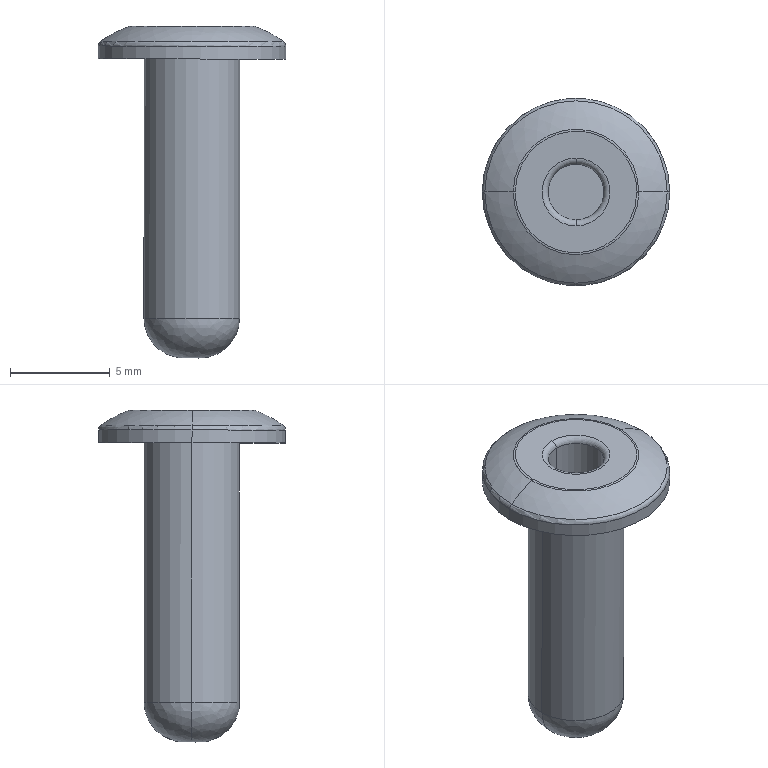Part | SolidWorks | features BaseBody 1 | 1 solid | 22 faces | box 9.401 x 9.4 x 16.653 mm | volume 328.564 mm3 | torus 8 | cylinder 6 | spline 4 | plane 4 | commonest cylinder face diameters 2.8 x2 4.8 x2 9.4 x2
STEP:
#1=CARTESIAN_POINT('',(200.964,12.529,-10.322));
#2=VERTEX_POINT('',#1);
#3=CARTESIAN_POINT('',(200.837,12.529,-10.077));
#4=VERTEX_POINT('',#3);
#5=CARTESIAN_POINT('',(200.664,12.529,-10.322));
#6=DIRECTION('',(0.00003827,-1.,-0.0004455));
#7=DIRECTION('',(1.,0.00003864,-0.0008339));
#8=AXIS2_PLACEMENT_3D('',#5,#6,#7);
#9=CIRCLE('',#8,0.3);
#10=EDGE_CURVE('',#2,#4,#9,.T.);
#11=ORIENTED_EDGE('',*,*,#10,.T.);
#12=CARTESIAN_POINT('',(191.692,12.529,-10.069));
#13=VERTEX_POINT('',#12);
#14=CARTESIAN_POINT('',(196.265,12.529,-10.073));
#15=DIRECTION('',(-0.0008339,0.0004454,-1.));
#16=DIRECTION('',(1.,0.00002965,-0.0008339));
#17=AXIS2_PLACEMENT_3D('',#14,#15,#16);
#18=CIRCLE('',#17,4.573);
#19=EDGE_CURVE('',#4,#13,#18,.T.);
#20=ORIENTED_EDGE('',*,*,#19,.T.);
#21=CARTESIAN_POINT('',(191.564,12.529,-10.315));
#22=VERTEX_POINT('',#21);
#23=CARTESIAN_POINT('',(191.864,12.529,-10.315));
#24=DIRECTION('',(-0.00003827,1.,0.0004455));
#25=DIRECTION('',(-1.,-0.00003864,0.0008339));
#26=AXIS2_PLACEMENT_3D('',#23,#24,#25);
#27=CIRCLE('',#26,0.3);
#28=EDGE_CURVE('',#22,#13,#27,.T.);
#29=ORIENTED_EDGE('',*,*,#28,.F.);
#30=CARTESIAN_POINT('',(196.264,12.529,-10.318));
#31=DIRECTION('',(-0.0008339,0.0004454,-1.));
#32=DIRECTION('',(-1.,-0.007345,0.0008306));
#33=AXIS2_PLACEMENT_3D('',#30,#31,#32);
#34=CIRCLE('',#33,4.7);
#35=EDGE_CURVE('',#2,#22,#34,.T.);
#36=ORIENTED_EDGE('',*,*,#35,.F.);
#37=EDGE_LOOP('',(#11,#20,#29,#36));
#38=FACE_OUTER_BOUND('',#37,.T.);
#39=CARTESIAN_POINT('',(196.264,12.529,-10.318));
#40=DIRECTION('',(-0.0008339,0.0004454,-1.));
#41=DIRECTION('',(1.,0.007345,-0.0008306));
#42=AXIS2_PLACEMENT_3D('',#39,#40,#41);
#43=TOROIDAL_SURFACE('',#42,4.4,0.3);
#44=ADVANCED_FACE('',(#38),#43,.T.);
#45=CARTESIAN_POINT('',(191.564,12.529,-10.961));
#46=VERTEX_POINT('',#45);
#47=CARTESIAN_POINT('',(200.964,12.529,-10.969));
#48=VERTEX_POINT('',#47);
#49=CARTESIAN_POINT('',(196.264,12.529,-10.965));
#50=DIRECTION('',(0.0008339,-0.0004454,1.));
#51=DIRECTION('',(-1.,-0.00003864,0.0008339));
#52=AXIS2_PLACEMENT_3D('',#49,#50,#51);
#53=CIRCLE('',#52,4.7);
#54=EDGE_CURVE('',#46,#48,#53,.T.);
#55=ORIENTED_EDGE('',*,*,#54,.T.);
#56=CARTESIAN_POINT('',(200.964,12.529,-10.322));
#57=DIRECTION('',(-0.0008339,0.0004454,-1.));
#58=VECTOR('',#57,1000.);
#59=LINE('',#56,#58);
#60=EDGE_CURVE('',#2,#48,#59,.T.);
#61=ORIENTED_EDGE('',*,*,#60,.F.);
#62=ORIENTED_EDGE('',*,*,#35,.T.);
#63=CARTESIAN_POINT('',(191.564,12.529,-10.315));
#64=DIRECTION('',(-0.0008339,0.0004454,-1.));
#65=VECTOR('',#64,1000.);
#66=LINE('',#63,#65);
#67=EDGE_CURVE('',#22,#46,#66,.T.);
#68=ORIENTED_EDGE('',*,*,#67,.T.);
#69=EDGE_LOOP('',(#55,#61,#62,#68));
#70=FACE_OUTER_BOUND('',#69,.T.);
#71=CARTESIAN_POINT('',(196.265,12.529,-9.315));
#72=DIRECTION('',(-0.0008339,0.0004454,-1.));
#73=DIRECTION('',(1.,0.00003864,-0.0008339));
#74=AXIS2_PLACEMENT_3D('',#71,#72,#73);
#75=CYLINDRICAL_SURFACE('',#74,4.7);
#76=ADVANCED_FACE('',(#70),#75,.T.);
#77=CARTESIAN_POINT('',(196.264,12.529,-10.965));
#78=DIRECTION('',(0.0008339,-0.0004454,1.));
#79=DIRECTION('',(1.,0.00003864,-0.0008339));
#80=AXIS2_PLACEMENT_3D('',#77,#78,#79);
#81=CIRCLE('',#80,4.7);
#82=EDGE_CURVE('',#48,#46,#81,.T.);
#83=ORIENTED_EDGE('',*,*,#82,.T.);
#84=ORIENTED_EDGE('',*,*,#67,.F.);
#85=CARTESIAN_POINT('',(196.264,12.529,-10.318));
#86=DIRECTION('',(-0.0008339,0.0004454,-1.));
#87=DIRECTION('',(-1.,-0.00003864,0.0008339));
#88=AXIS2_PLACEMENT_3D('',#85,#86,#87);
#89=CIRCLE('',#88,4.7);
#90=EDGE_CURVE('',#22,#2,#89,.T.);
#91=ORIENTED_EDGE('',*,*,#90,.T.);
#92=ORIENTED_EDGE('',*,*,#60,.T.);
#93=EDGE_LOOP('',(#83,#84,#91,#92));
#94=FACE_OUTER_BOUND('',#93,.T.);
#95=CARTESIAN_POINT('',(196.265,12.529,-9.315));
#96=DIRECTION('',(-0.0008339,0.0004454,-1.));
#97=DIRECTION('',(1.,0.00003864,-0.0008339));
#98=AXIS2_PLACEMENT_3D('',#95,#96,#97);
#99=CYLINDRICAL_SURFACE('',#98,4.7);
#100=ADVANCED_FACE('',(#94),#99,.T.);
#101=ORIENTED_EDGE('',*,*,#28,.T.);
#102=CARTESIAN_POINT('',(196.265,12.529,-10.073));
#103=DIRECTION('',(-0.0008339,0.0004454,-1.));
#104=DIRECTION('',(-1.,-0.00002965,0.0008339));
#105=AXIS2_PLACEMENT_3D('',#102,#103,#104);
#106=CIRCLE('',#105,4.573);
#107=EDGE_CURVE('',#13,#4,#106,.T.);
#108=ORIENTED_EDGE('',*,*,#107,.T.);
#109=ORIENTED_EDGE('',*,*,#10,.F.);
#110=ORIENTED_EDGE('',*,*,#90,.F.);
#111=EDGE_LOOP('',(#101,#108,#109,#110));
#112=FACE_OUTER_BOUND('',#111,.T.);
#113=CARTESIAN_POINT('',(196.264,12.529,-10.318));
#114=DIRECTION('',(-0.0008339,0.0004454,-1.));
#115=DIRECTION('',(-1.,-0.007345,0.0008306));
#116=AXIS2_PLACEMENT_3D('',#113,#114,#115);
#117=TOROIDAL_SURFACE('',#116,4.4,0.3);
#118=ADVANCED_FACE('',(#112),#117,.T.);
#119=CARTESIAN_POINT('',(199.415,12.529,-9.336));
#120=VERTEX_POINT('',#119);
#121=CARTESIAN_POINT('',(200.837,12.529,-10.077));
#122=CARTESIAN_POINT('',(200.691,12.529,-9.974));
#123=CARTESIAN_POINT('',(200.39,12.529,-9.781));
#124=CARTESIAN_POINT('',(199.915,12.529,-9.533));
#125=CARTESIAN_POINT('',(199.584,12.529,-9.396));
#126=CARTESIAN_POINT('',(199.415,12.529,-9.336));
#127=B_SPLINE_CURVE_WITH_KNOTS('',3,(#121,#122,#123,#124,#125,#126),.UNSPECIFIED.,.F.,.F.,(4,1,1,4),(0.000000006,0.3333,0.6667,1.),.UNSPECIFIED.);
#128=EDGE_CURVE('',#4,#120,#127,.T.);
#129=ORIENTED_EDGE('',*,*,#128,.F.);
#130=ORIENTED_EDGE('',*,*,#107,.F.);
#131=CARTESIAN_POINT('',(193.115,12.528,-9.33));
#132=VERTEX_POINT('',#131);
#133=CARTESIAN_POINT('',(191.692,12.529,-10.069));
#134=CARTESIAN_POINT('',(191.838,12.529,-9.967));
#135=CARTESIAN_POINT('',(192.139,12.529,-9.774));
#136=CARTESIAN_POINT('',(192.616,12.529,-9.527));
#137=CARTESIAN_POINT('',(192.947,12.528,-9.391));
#138=CARTESIAN_POINT('',(193.115,12.528,-9.33));
#139=B_SPLINE_CURVE_WITH_KNOTS('',3,(#133,#134,#135,#136,#137,#138),.UNSPECIFIED.,.F.,.F.,(4,1,1,4),(0.000001822,0.3333,0.6667,1.),.UNSPECIFIED.);
#140=EDGE_CURVE('',#13,#132,#139,.T.);
#141=ORIENTED_EDGE('',*,*,#140,.T.);
#142=CARTESIAN_POINT('',(193.116,12.566,-9.33));
#143=VERTEX_POINT('',#142);
#144=CARTESIAN_POINT('',(196.265,12.529,-9.333));
#145=DIRECTION('',(0.0008339,-0.0004454,1.));
#146=DIRECTION('',(-0.9999,0.01201,0.0008392));
#147=AXIS2_PLACEMENT_3D('',#144,#145,#146);
#148=CIRCLE('',#147,3.15);
#149=EDGE_CURVE('',#143,#132,#148,.T.);
#150=ORIENTED_EDGE('',*,*,#149,.F.);
#151=CARTESIAN_POINT('',(196.265,12.529,-9.333));
#152=DIRECTION('',(0.0008339,-0.0004454,1.));
#153=DIRECTION('',(-0.9999,0.01201,0.0008392));
#154=AXIS2_PLACEMENT_3D('',#151,#152,#153);
#155=CIRCLE('',#154,3.15);
#156=EDGE_CURVE('',#120,#143,#155,.T.);
#157=ORIENTED_EDGE('',*,*,#156,.F.);
#158=EDGE_LOOP('',(#129,#130,#141,#150,#157));
#159=FACE_OUTER_BOUND('',#158,.T.);
#160=CARTESIAN_POINT('',(193.235,12.338,-9.291));
#161=CARTESIAN_POINT('',(192.65,12.301,-9.489));
#162=CARTESIAN_POINT('',(192.102,12.267,-9.774));
#163=CARTESIAN_POINT('',(191.604,12.235,-10.14));
#164=CARTESIAN_POINT('',(193.117,14.203,-9.29));
#165=CARTESIAN_POINT('',(192.509,14.526,-9.487));
#166=CARTESIAN_POINT('',(191.94,14.829,-9.772));
#167=CARTESIAN_POINT('',(191.423,15.104,-10.138));
#168=CARTESIAN_POINT('',(194.396,15.565,-9.291));
#169=CARTESIAN_POINT('',(194.036,16.151,-9.488));
#170=CARTESIAN_POINT('',(193.698,16.7,-9.773));
#171=CARTESIAN_POINT('',(193.39,17.199,-10.139));
#172=CARTESIAN_POINT('',(196.265,15.565,-9.292));
#173=CARTESIAN_POINT('',(196.265,16.151,-9.49));
#174=CARTESIAN_POINT('',(196.265,16.7,-9.775));
#175=CARTESIAN_POINT('',(196.264,17.199,-10.141));
#176=CARTESIAN_POINT('',(198.134,15.565,-9.294));
#177=CARTESIAN_POINT('',(198.495,16.151,-9.492));
#178=CARTESIAN_POINT('',(198.832,16.7,-9.777));
#179=CARTESIAN_POINT('',(199.138,17.199,-10.144));
#180=CARTESIAN_POINT('',(199.413,14.203,-9.295));
#181=CARTESIAN_POINT('',(200.021,14.526,-9.494));
#182=CARTESIAN_POINT('',(200.589,14.829,-9.78));
#183=CARTESIAN_POINT('',(201.106,15.104,-10.146));
#184=CARTESIAN_POINT('',(199.296,12.338,-9.296));
#185=CARTESIAN_POINT('',(199.881,12.301,-9.495));
#186=CARTESIAN_POINT('',(200.428,12.267,-9.781));
#187=CARTESIAN_POINT('',(200.926,12.236,-10.147));
#188=(BOUNDED_SURFACE()B_SPLINE_SURFACE(3,3,((#160,#161,#162,#163),(#164,#165,#166,#167),(#168,#169,#170,#171),(#172,#173,#174,#175),(#176,#177,#178,#179),(#180,#181,#182,#183),(#184,#185,#186,#187)),.UNSPECIFIED.,.F.,.F.,.F.)B_SPLINE_SURFACE_WITH_KNOTS((4,3,4),(4,4),(0.,1.,2.),(0.,1.),.UNSPECIFIED.)GEOMETRIC_REPRESENTATION_ITEM()RATIONAL_B_SPLINE_SURFACE(((1.194,1.185,1.185,1.194),(0.9432,0.9357,0.9357,0.9432),(0.9432,0.9357,0.9357,0.9432),(1.194,1.185,1.185,1.194),(0.9432,0.9357,0.9357,0.9432),(0.9432,0.9357,0.9357,0.9432),(1.194,1.185,1.185,1.194)))REPRESENTATION_ITEM('')SURFACE());
#189=ADVANCED_FACE('',(#159),#188,.T.);
#190=CARTESIAN_POINT('',(193.216,12.565,-9.313));
#191=VERTEX_POINT('',#190);
#192=CARTESIAN_POINT('',(193.217,12.565,-9.613));
#193=DIRECTION('',(-0.01201,-0.9999,-0.0004354));
#194=DIRECTION('',(0.9999,-0.01201,0.));
#195=AXIS2_PLACEMENT_3D('',#192,#193,#194);
#196=CIRCLE('',#195,0.3);
#197=EDGE_CURVE('',#191,#143,#196,.T.);
#198=ORIENTED_EDGE('',*,*,#197,.F.);
#199=CARTESIAN_POINT('',(199.315,12.527,-9.318));
#200=VERTEX_POINT('',#199);
#201=CARTESIAN_POINT('',(193.216,12.565,-9.313));
#202=CARTESIAN_POINT('',(193.221,12.711,-9.313));
#203=CARTESIAN_POINT('',(193.234,12.911,-9.313));
#204=CARTESIAN_POINT('',(193.298,13.218,-9.313));
#205=CARTESIAN_POINT('',(193.313,13.284,-9.313));
#206=CARTESIAN_POINT('',(193.345,13.401,-9.313));
#207=CARTESIAN_POINT('',(193.362,13.456,-9.313));
#208=CARTESIAN_POINT('',(193.414,13.612,-9.313));
#209=CARTESIAN_POINT('',(193.45,13.702,-9.313));
#210=CARTESIAN_POINT('',(193.502,13.817,-9.312));
#211=CARTESIAN_POINT('',(193.519,13.853,-9.312));
#212=CARTESIAN_POINT('',(193.539,13.893,-9.312));
#213=CARTESIAN_POINT('',(193.543,13.902,-9.312));
#214=CARTESIAN_POINT('',(193.554,13.924,-9.312));
#215=CARTESIAN_POINT('',(193.571,13.956,-9.312));
#216=CARTESIAN_POINT('',(193.635,14.074,-9.312));
#217=CARTESIAN_POINT('',(193.699,14.178,-9.312));
#218=CARTESIAN_POINT('',(193.783,14.299,-9.313));
#219=CARTESIAN_POINT('',(193.826,14.358,-9.313));
#220=CARTESIAN_POINT('',(193.871,14.416,-9.313));
#221=CARTESIAN_POINT('',(193.894,14.444,-9.313));
#222=CARTESIAN_POINT('',(193.904,14.456,-9.313));
#223=CARTESIAN_POINT('',(193.913,14.467,-9.313));
#224=CARTESIAN_POINT('',(193.917,14.472,-9.313));
#225=CARTESIAN_POINT('',(193.961,14.524,-9.313));
#226=CARTESIAN_POINT('',(194.013,14.584,-9.313));
#227=CARTESIAN_POINT('',(194.149,14.724,-9.313));
#228=CARTESIAN_POINT('',(194.233,14.804,-9.313));
#229=CARTESIAN_POINT('',(194.351,14.9,-9.313));
#230=CARTESIAN_POINT('',(194.365,14.911,-9.313));
#231=CARTESIAN_POINT('',(194.385,14.927,-9.313));
#232=CARTESIAN_POINT('',(194.389,14.93,-9.313));
#233=CARTESIAN_POINT('',(194.398,14.937,-9.313));
#234=CARTESIAN_POINT('',(194.42,14.954,-9.313));
#235=CARTESIAN_POINT('',(194.477,14.997,-9.313));
#236=CARTESIAN_POINT('',(194.533,15.036,-9.313));
#237=CARTESIAN_POINT('',(194.724,15.165,-9.313));
#238=CARTESIAN_POINT('',(194.897,15.26,-9.313));
#239=CARTESIAN_POINT('',(195.135,15.36,-9.313));
#240=CARTESIAN_POINT('',(195.184,15.38,-9.313));
#241=CARTESIAN_POINT('',(195.241,15.4,-9.313));
#242=CARTESIAN_POINT('',(195.247,15.402,-9.313));
#243=CARTESIAN_POINT('',(195.26,15.407,-9.313));
#244=CARTESIAN_POINT('',(195.258,15.406,-9.313));
#245=CARTESIAN_POINT('',(195.263,15.408,-9.313));
#246=CARTESIAN_POINT('',(195.275,15.412,-9.313));
#247=CARTESIAN_POINT('',(195.293,15.418,-9.313));
#248=CARTESIAN_POINT('',(195.364,15.442,-9.313));
#249=CARTESIAN_POINT('',(195.464,15.474,-9.313));
#250=CARTESIAN_POINT('',(195.679,15.521,-9.314));
#251=CARTESIAN_POINT('',(195.768,15.537,-9.314));
#252=CARTESIAN_POINT('',(195.914,15.557,-9.314));
#253=CARTESIAN_POINT('',(195.979,15.563,-9.314));
#254=CARTESIAN_POINT('',(196.088,15.571,-9.314));
#255=CARTESIAN_POINT('',(196.133,15.573,-9.314));
#256=CARTESIAN_POINT('',(196.186,15.575,-9.314));
#257=CARTESIAN_POINT('',(196.201,15.575,-9.314));
#258=CARTESIAN_POINT('',(196.227,15.576,-9.314));
#259=CARTESIAN_POINT('',(196.238,15.576,-9.314));
#260=CARTESIAN_POINT('',(196.273,15.576,-9.314));
#261=CARTESIAN_POINT('',(196.336,15.577,-9.314));
#262=CARTESIAN_POINT('',(196.484,15.569,-9.314));
#263=CARTESIAN_POINT('',(196.542,15.564,-9.314));
#264=CARTESIAN_POINT('',(196.643,15.553,-9.314));
#265=CARTESIAN_POINT('',(196.678,15.549,-9.314));
#266=CARTESIAN_POINT('',(196.735,15.54,-9.314));
#267=CARTESIAN_POINT('',(196.764,15.536,-9.314));
#268=CARTESIAN_POINT('',(196.799,15.53,-9.314));
#269=CARTESIAN_POINT('',(196.817,15.526,-9.314));
#270=CARTESIAN_POINT('',(196.825,15.525,-9.315));
#271=CARTESIAN_POINT('',(196.83,15.524,-9.315));
#272=CARTESIAN_POINT('',(196.834,15.523,-9.315));
#273=CARTESIAN_POINT('',(196.93,15.505,-9.315));
#274=CARTESIAN_POINT('',(197.025,15.483,-9.315));
#275=CARTESIAN_POINT('',(197.167,15.441,-9.315));
#276=CARTESIAN_POINT('',(197.238,15.419,-9.315));
#277=CARTESIAN_POINT('',(197.32,15.389,-9.315));
#278=CARTESIAN_POINT('',(197.361,15.373,-9.315));
#279=CARTESIAN_POINT('',(197.382,15.365,-9.315));
#280=CARTESIAN_POINT('',(197.392,15.361,-9.315));
#281=CARTESIAN_POINT('',(197.397,15.36,-9.315));
#282=CARTESIAN_POINT('',(197.399,15.358,-9.315));
#283=CARTESIAN_POINT('',(197.4,15.358,-9.315));
#284=CARTESIAN_POINT('',(197.581,15.285,-9.315));
#285=CARTESIAN_POINT('',(197.731,15.205,-9.315));
#286=CARTESIAN_POINT('',(197.981,15.052,-9.316));
#287=CARTESIAN_POINT('',(198.081,14.979,-9.316));
#288=CARTESIAN_POINT('',(198.237,14.855,-9.316));
#289=CARTESIAN_POINT('',(198.294,14.804,-9.316));
#290=CARTESIAN_POINT('',(198.354,14.749,-9.316));
#291=CARTESIAN_POINT('',(198.369,14.735,-9.316));
#292=CARTESIAN_POINT('',(198.385,14.719,-9.316));
#293=CARTESIAN_POINT('',(198.392,14.712,-9.316));
#294=CARTESIAN_POINT('',(198.397,14.707,-9.316));
#295=CARTESIAN_POINT('',(198.399,14.706,-9.316));
#296=CARTESIAN_POINT('',(198.399,14.705,-9.316));
#297=CARTESIAN_POINT('',(198.4,14.705,-9.316));
#298=CARTESIAN_POINT('',(198.398,14.706,-9.316));
#299=CARTESIAN_POINT('',(198.453,14.653,-9.316));
#300=CARTESIAN_POINT('',(198.514,14.589,-9.316));
#301=CARTESIAN_POINT('',(198.612,14.474,-9.316));
#302=CARTESIAN_POINT('',(198.646,14.432,-9.317));
#303=CARTESIAN_POINT('',(198.699,14.364,-9.317));
#304=CARTESIAN_POINT('',(198.725,14.329,-9.317));
#305=CARTESIAN_POINT('',(198.757,14.285,-9.317));
#306=CARTESIAN_POINT('',(198.772,14.262,-9.317));
#307=CARTESIAN_POINT('',(198.779,14.252,-9.317));
#308=CARTESIAN_POINT('',(198.784,14.246,-9.317));
#309=CARTESIAN_POINT('',(198.787,14.241,-9.317));
#310=CARTESIAN_POINT('',(198.837,14.166,-9.317));
#311=CARTESIAN_POINT('',(198.887,14.086,-9.317));
#312=CARTESIAN_POINT('',(198.96,13.954,-9.317));
#313=CARTESIAN_POINT('',(198.984,13.908,-9.317));
#314=CARTESIAN_POINT('',(199.019,13.835,-9.317));
#315=CARTESIAN_POINT('',(199.031,13.811,-9.317));
#316=CARTESIAN_POINT('',(199.054,13.76,-9.317));
#317=CARTESIAN_POINT('',(199.066,13.733,-9.317));
#318=CARTESIAN_POINT('',(199.117,13.61,-9.317));
#319=CARTESIAN_POINT('',(199.152,13.513,-9.317));
#320=CARTESIAN_POINT('',(199.196,13.37,-9.317));
#321=CARTESIAN_POINT('',(199.215,13.299,-9.317));
#322=CARTESIAN_POINT('',(199.235,13.218,-9.318));
#323=CARTESIAN_POINT('',(199.244,13.178,-9.318));
#324=CARTESIAN_POINT('',(199.248,13.158,-9.318));
#325=CARTESIAN_POINT('',(199.25,13.149,-9.318));
#326=CARTESIAN_POINT('',(199.251,13.143,-9.318));
#327=CARTESIAN_POINT('',(199.252,13.139,-9.318));
#328=CARTESIAN_POINT('',(199.257,13.114,-9.318));
#329=CARTESIAN_POINT('',(199.265,13.072,-9.318));
#330=CARTESIAN_POINT('',(199.28,12.981,-9.318));
#331=CARTESIAN_POINT('',(199.285,12.946,-9.318));
#332=CARTESIAN_POINT('',(199.293,12.886,-9.318));
#333=CARTESIAN_POINT('',(199.296,12.854,-9.318));
#334=CARTESIAN_POINT('',(199.3,12.814,-9.318));
#335=CARTESIAN_POINT('',(199.302,12.796,-9.318));
#336=CARTESIAN_POINT('',(199.303,12.784,-9.318));
#337=CARTESIAN_POINT('',(199.304,12.776,-9.318));
#338=CARTESIAN_POINT('',(199.316,12.631,-9.318));
#339=CARTESIAN_POINT('',(199.314,12.549,-9.318));
#340=CARTESIAN_POINT('',(199.315,12.527,-9.318));
#341=B_SPLINE_CURVE_WITH_KNOTS('',3,(#201,#202,#203,#204,#205,#206,#207,#208,#209,#210,#211,#212,#213,#214,#215,#216,#217,#218,#219,#220,#221,#222,#223,#224,#225,#226,#227,#228,#229,#230,#231,#232,#233,#234,#235,#236,#237,#238,#239,#240,#241,#242,#243,#244,#245,#246,#247,#248,#249,#250,#251,#252,#253,#254,#255,#256,#257,#258,#259,#260,#261,#262,#263,#264,#265,#266,#267,#268,#269,#270,#271,#272,#273,#274,#275,#276,#277,#278,#279,#280,#281,#282,#283,#284,#285,#286,#287,#288,#289,#290,#291,#292,#293,#294,#295,#296,#297,#298,#299,#300,#301,#302,#303,#304,#305,#306,#307,#308,#309,#310,#311,#312,#313,#314,#315,#316,#317,#318,#319,#320,#321,#322,#323,#324,#325,#326,#327,#328,#329,#330,#331,#332,#333,#334,#335,#336,#337,#338,#339,#340),.UNSPECIFIED.,.F.,.F.,(4,2,2,2,2,2,2,1,1,2,1,2,2,2,2,2,2,2,1,1,2,2,2,2,2,1,2,2,2,2,2,2,2,2,2,2,1,1,1,2,2,2,1,1,1,1,1,2,2,2,2,2,2,1,1,1,2,2,2,2,1,1,1,2,2,2,2,2,2,2,1,1,1,1,2,2,2,2,1,1,2,2,4),(0.,0.0625,0.07813,0.09375,0.125,0.1406,0.1445,0.1484,0.1563,0.1875,0.2031,0.2109,0.2148,0.2188,0.25,0.2813,0.2852,0.2871,0.2891,0.2969,0.3125,0.375,0.3906,0.3926,0.3945,0.3984,0.4063,0.4375,0.4531,0.4688,0.4844,0.4922,0.5,0.5313,0.5469,0.5547,0.5586,0.5605,0.5615,0.562,0.5625,0.5938,0.6094,0.6172,0.6211,0.623,0.624,0.6245,0.625,0.6563,0.6875,0.7188,0.7344,0.7422,0.7461,0.748,0.749,0.75,0.7813,0.7969,0.8047,0.8086,0.8105,0.8115,0.8125,0.8438,0.8594,0.8672,0.875,0.9063,0.9219,0.9297,0.9336,0.9355,0.9365,0.9375,0.9531,0.9609,0.9648,0.9668,0.9678,0.9688,1.),.UNSPECIFIED.);
#342=EDGE_CURVE('',#191,#200,#341,.T.);
#343=ORIENTED_EDGE('',*,*,#342,.T.);
#344=CARTESIAN_POINT('',(199.313,12.529,-9.618));
#345=DIRECTION('',(-0.00003827,1.,0.0004455));
#346=DIRECTION('',(0.004566,-0.0004453,1.));
#347=AXIS2_PLACEMENT_3D('',#344,#345,#346);
#348=CIRCLE('',#347,0.3);
#349=EDGE_CURVE('',#200,#120,#348,.T.);
#350=ORIENTED_EDGE('',*,*,#349,.T.);
#351=ORIENTED_EDGE('',*,*,#156,.T.);
#352=EDGE_LOOP('',(#198,#343,#350,#351));
#353=FACE_OUTER_BOUND('',#352,.T.);
#354=CARTESIAN_POINT('',(196.265,12.529,-9.615));
#355=DIRECTION('',(-0.0008339,0.0004454,-1.));
#356=DIRECTION('',(0.9999,-0.01201,-0.0008392));
#357=AXIS2_PLACEMENT_3D('',#354,#355,#356);
#358=TOROIDAL_SURFACE('',#357,3.048,0.3);
#359=ADVANCED_FACE('',(#353),#358,.T.);
#360=CARTESIAN_POINT('',(196.262,14.23,-9.315));
#361=VERTEX_POINT('',#360);
#362=CARTESIAN_POINT('',(196.269,10.827,-9.316));
#363=VERTEX_POINT('',#362);
#364=CARTESIAN_POINT('',(196.262,14.23,-9.315));
#365=CARTESIAN_POINT('',(196.372,14.231,-9.315));
#366=CARTESIAN_POINT('',(196.479,14.222,-9.315));
#367=CARTESIAN_POINT('',(196.682,14.183,-9.315));
#368=CARTESIAN_POINT('',(196.782,14.154,-9.315));
#369=CARTESIAN_POINT('',(196.934,14.092,-9.315));
#370=CARTESIAN_POINT('',(196.984,14.069,-9.315));
#371=CARTESIAN_POINT('',(197.083,14.018,-9.315));
#372=CARTESIAN_POINT('',(197.13,13.991,-9.315));
#373=CARTESIAN_POINT('',(197.276,13.898,-9.316));
#374=CARTESIAN_POINT('',(197.366,13.828,-9.316));
#375=CARTESIAN_POINT('',(197.607,13.598,-9.316));
#376=CARTESIAN_POINT('',(197.739,13.405,-9.316));
#377=CARTESIAN_POINT('',(197.915,12.995,-9.317));
#378=CARTESIAN_POINT('',(197.963,12.77,-9.317));
#379=CARTESIAN_POINT('',(197.968,12.325,-9.317));
#380=CARTESIAN_POINT('',(197.924,12.097,-9.317));
#381=CARTESIAN_POINT('',(197.757,11.683,-9.317));
#382=CARTESIAN_POINT('',(197.628,11.488,-9.317));
#383=CARTESIAN_POINT('',(197.432,11.291,-9.317));
#384=CARTESIAN_POINT('',(197.391,11.253,-9.317));
#385=CARTESIAN_POINT('',(197.305,11.182,-9.317));
#386=CARTESIAN_POINT('',(197.258,11.148,-9.317));
#387=CARTESIAN_POINT('',(197.166,11.086,-9.317));
#388=CARTESIAN_POINT('',(197.118,11.057,-9.317));
#389=CARTESIAN_POINT('',(197.021,11.005,-9.317));
#390=CARTESIAN_POINT('',(196.969,10.98,-9.317));
#391=CARTESIAN_POINT('',(196.718,10.875,-9.316));
#392=CARTESIAN_POINT('',(196.502,10.831,-9.316));
#393=CARTESIAN_POINT('',(196.269,10.827,-9.316));
#394=B_SPLINE_CURVE_WITH_KNOTS('',3,(#364,#365,#366,#367,#368,#369,#370,#371,#372,#373,#374,#375,#376,#377,#378,#379,#380,#381,#382,#383,#384,#385,#386,#387,#388,#389,#390,#391,#392,#393),.UNSPECIFIED.,.F.,.F.,(4,2,2,2,2,2,2,2,2,2,2,2,2,2,4),(0.,0.0625,0.125,0.1562,0.1875,0.25,0.375,0.5,0.625,0.75,0.7812,0.8125,0.8437,0.875,1.),.UNSPECIFIED.);
#395=EDGE_CURVE('',#361,#363,#394,.T.);
#396=ORIENTED_EDGE('',*,*,#395,.T.);
#397=CARTESIAN_POINT('',(196.269,10.827,-9.316));
#398=CARTESIAN_POINT('',(196.159,10.826,-9.316));
#399=CARTESIAN_POINT('',(196.052,10.836,-9.316));
#400=CARTESIAN_POINT('',(195.849,10.874,-9.316));
#401=CARTESIAN_POINT('',(195.748,10.904,-9.316));
#402=CARTESIAN_POINT('',(195.596,10.965,-9.316));
#403=CARTESIAN_POINT('',(195.546,10.988,-9.315));
#404=CARTESIAN_POINT('',(195.448,11.039,-9.315));
#405=CARTESIAN_POINT('',(195.401,11.066,-9.315));
#406=CARTESIAN_POINT('',(195.255,11.159,-9.315));
#407=CARTESIAN_POINT('',(195.165,11.229,-9.315));
#408=CARTESIAN_POINT('',(194.924,11.459,-9.315));
#409=CARTESIAN_POINT('',(194.791,11.652,-9.315));
#410=CARTESIAN_POINT('',(194.616,12.062,-9.314));
#411=CARTESIAN_POINT('',(194.568,12.287,-9.314));
#412=CARTESIAN_POINT('',(194.563,12.733,-9.314));
#413=CARTESIAN_POINT('',(194.606,12.96,-9.314));
#414=CARTESIAN_POINT('',(194.774,13.374,-9.314));
#415=CARTESIAN_POINT('',(194.903,13.569,-9.314));
#416=CARTESIAN_POINT('',(195.098,13.766,-9.314));
#417=CARTESIAN_POINT('',(195.14,13.804,-9.314));
#418=CARTESIAN_POINT('',(195.226,13.875,-9.314));
#419=CARTESIAN_POINT('',(195.272,13.909,-9.314));
#420=CARTESIAN_POINT('',(195.365,13.971,-9.314));
#421=CARTESIAN_POINT('',(195.412,14.,-9.314));
#422=CARTESIAN_POINT('',(195.51,14.052,-9.314));
#423=CARTESIAN_POINT('',(195.561,14.077,-9.314));
#424=CARTESIAN_POINT('',(195.812,14.182,-9.314));
#425=CARTESIAN_POINT('',(196.029,14.226,-9.314));
#426=CARTESIAN_POINT('',(196.262,14.23,-9.315));
#427=B_SPLINE_CURVE_WITH_KNOTS('',3,(#397,#398,#399,#400,#401,#402,#403,#404,#405,#406,#407,#408,#409,#410,#411,#412,#413,#414,#415,#416,#417,#418,#419,#420,#421,#422,#423,#424,#425,#426),.UNSPECIFIED.,.F.,.F.,(4,2,2,2,2,2,2,2,2,2,2,2,2,2,4),(0.,0.0625,0.125,0.1562,0.1875,0.25,0.375,0.5,0.625,0.75,0.7813,0.8125,0.8438,0.875,1.),.UNSPECIFIED.);
#428=EDGE_CURVE('',#363,#361,#427,.T.);
#429=ORIENTED_EDGE('',*,*,#428,.T.);
#430=EDGE_LOOP('',(#396,#429));
#431=FACE_BOUND('',#430,.T.);
#432=CARTESIAN_POINT('',(199.315,12.492,-9.318));
#433=VERTEX_POINT('',#432);
#434=CARTESIAN_POINT('',(193.216,12.53,-9.313));
#435=VERTEX_POINT('',#434);
#436=CARTESIAN_POINT('',(199.315,12.492,-9.318));
#437=CARTESIAN_POINT('',(199.309,12.346,-9.318));
#438=CARTESIAN_POINT('',(199.296,12.146,-9.318));
#439=CARTESIAN_POINT('',(199.233,11.839,-9.318));
#440=CARTESIAN_POINT('',(199.217,11.774,-9.318));
#441=CARTESIAN_POINT('',(199.185,11.656,-9.318));
#442=CARTESIAN_POINT('',(199.169,11.601,-9.318));
#443=CARTESIAN_POINT('',(199.117,11.445,-9.318));
#444=CARTESIAN_POINT('',(199.08,11.355,-9.318));
#445=CARTESIAN_POINT('',(199.029,11.24,-9.318));
#446=CARTESIAN_POINT('',(199.012,11.204,-9.318));
#447=CARTESIAN_POINT('',(198.992,11.164,-9.318));
#448=CARTESIAN_POINT('',(198.988,11.155,-9.318));
#449=CARTESIAN_POINT('',(198.977,11.134,-9.318));
#450=CARTESIAN_POINT('',(198.96,11.101,-9.318));
#451=CARTESIAN_POINT('',(198.896,10.983,-9.318));
#452=CARTESIAN_POINT('',(198.831,10.879,-9.318));
#453=CARTESIAN_POINT('',(198.748,10.758,-9.318));
#454=CARTESIAN_POINT('',(198.705,10.699,-9.318));
#455=CARTESIAN_POINT('',(198.66,10.641,-9.318));
#456=CARTESIAN_POINT('',(198.637,10.613,-9.318));
#457=CARTESIAN_POINT('',(198.627,10.601,-9.318));
#458=CARTESIAN_POINT('',(198.618,10.59,-9.318));
#459=CARTESIAN_POINT('',(198.613,10.585,-9.318));
#460=CARTESIAN_POINT('',(198.57,10.533,-9.318));
#461=CARTESIAN_POINT('',(198.518,10.473,-9.318));
#462=CARTESIAN_POINT('',(198.382,10.333,-9.318));
#463=CARTESIAN_POINT('',(198.297,10.253,-9.318));
#464=CARTESIAN_POINT('',(198.179,10.157,-9.318));
#465=CARTESIAN_POINT('',(198.166,10.146,-9.318));
#466=CARTESIAN_POINT('',(198.145,10.13,-9.318));
#467=CARTESIAN_POINT('',(198.141,10.127,-9.318));
#468=CARTESIAN_POINT('',(198.133,10.12,-9.318));
#469=CARTESIAN_POINT('',(198.111,10.103,-9.318));
#470=CARTESIAN_POINT('',(198.053,10.06,-9.318));
#471=CARTESIAN_POINT('',(197.998,10.021,-9.318));
#472=CARTESIAN_POINT('',(197.806,9.892,-9.318));
#473=CARTESIAN_POINT('',(197.634,9.797,-9.318));
#474=CARTESIAN_POINT('',(197.395,9.697,-9.318));
#475=CARTESIAN_POINT('',(197.346,9.678,-9.318));
#476=CARTESIAN_POINT('',(197.29,9.657,-9.318));
#477=CARTESIAN_POINT('',(197.284,9.655,-9.318));
#478=CARTESIAN_POINT('',(197.271,9.65,-9.317));
#479=CARTESIAN_POINT('',(197.272,9.651,-9.317));
#480=CARTESIAN_POINT('',(197.267,9.649,-9.317));
#481=CARTESIAN_POINT('',(197.256,9.645,-9.317));
#482=CARTESIAN_POINT('',(197.238,9.639,-9.317));
#483=CARTESIAN_POINT('',(197.166,9.615,-9.317));
#484=CARTESIAN_POINT('',(197.067,9.584,-9.317));
#485=CARTESIAN_POINT('',(196.851,9.536,-9.317));
#486=CARTESIAN_POINT('',(196.763,9.52,-9.317));
#487=CARTESIAN_POINT('',(196.616,9.5,-9.317));
#488=CARTESIAN_POINT('',(196.552,9.494,-9.317));
#489=CARTESIAN_POINT('',(196.443,9.486,-9.317));
#490=CARTESIAN_POINT('',(196.398,9.484,-9.317));
#491=CARTESIAN_POINT('',(196.345,9.482,-9.317));
#492=CARTESIAN_POINT('',(196.33,9.482,-9.317));
#493=CARTESIAN_POINT('',(196.304,9.481,-9.317));
#494=CARTESIAN_POINT('',(196.292,9.481,-9.317));
#495=CARTESIAN_POINT('',(196.258,9.481,-9.317));
#496=CARTESIAN_POINT('',(196.194,9.48,-9.317));
#497=CARTESIAN_POINT('',(196.046,9.488,-9.317));
#498=CARTESIAN_POINT('',(195.988,9.493,-9.316));
#499=CARTESIAN_POINT('',(195.888,9.504,-9.316));
#500=CARTESIAN_POINT('',(195.852,9.508,-9.316));
#501=CARTESIAN_POINT('',(195.796,9.517,-9.316));
#502=CARTESIAN_POINT('',(195.767,9.521,-9.316));
#503=CARTESIAN_POINT('',(195.732,9.527,-9.316));
#504=CARTESIAN_POINT('',(195.714,9.531,-9.316));
#505=CARTESIAN_POINT('',(195.706,9.532,-9.316));
#506=CARTESIAN_POINT('',(195.701,9.533,-9.316));
#507=CARTESIAN_POINT('',(195.697,9.534,-9.316));
#508=CARTESIAN_POINT('',(195.601,9.552,-9.316));
#509=CARTESIAN_POINT('',(195.506,9.574,-9.316));
#510=CARTESIAN_POINT('',(195.364,9.616,-9.316));
#511=CARTESIAN_POINT('',(195.293,9.638,-9.316));
#512=CARTESIAN_POINT('',(195.21,9.668,-9.316));
#513=CARTESIAN_POINT('',(195.169,9.684,-9.316));
#514=CARTESIAN_POINT('',(195.149,9.692,-9.316));
#515=CARTESIAN_POINT('',(195.138,9.696,-9.316));
#516=CARTESIAN_POINT('',(195.134,9.698,-9.316));
#517=CARTESIAN_POINT('',(195.131,9.699,-9.316));
#518=CARTESIAN_POINT('',(195.131,9.699,-9.316));
#519=CARTESIAN_POINT('',(194.949,9.772,-9.316));
#520=CARTESIAN_POINT('',(194.799,9.852,-9.315));
#521=CARTESIAN_POINT('',(194.55,10.005,-9.315));
#522=CARTESIAN_POINT('',(194.45,10.078,-9.315));
#523=CARTESIAN_POINT('',(194.293,10.202,-9.315));
#524=CARTESIAN_POINT('',(194.236,10.253,-9.315));
#525=CARTESIAN_POINT('',(194.177,10.308,-9.315));
#526=CARTESIAN_POINT('',(194.162,10.322,-9.315));
#527=CARTESIAN_POINT('',(194.145,10.338,-9.315));
#528=CARTESIAN_POINT('',(194.139,10.345,-9.315));
#529=CARTESIAN_POINT('',(194.134,10.35,-9.315));
#530=CARTESIAN_POINT('',(194.132,10.351,-9.315));
#531=CARTESIAN_POINT('',(194.131,10.352,-9.315));
#532=CARTESIAN_POINT('',(194.131,10.352,-9.315));
#533=CARTESIAN_POINT('',(194.132,10.351,-9.315));
#534=CARTESIAN_POINT('',(194.078,10.405,-9.314));
#535=CARTESIAN_POINT('',(194.017,10.468,-9.314));
#536=CARTESIAN_POINT('',(193.918,10.583,-9.314));
#537=CARTESIAN_POINT('',(193.884,10.625,-9.314));
#538=CARTESIAN_POINT('',(193.832,10.693,-9.314));
#539=CARTESIAN_POINT('',(193.805,10.728,-9.314));
#540=CARTESIAN_POINT('',(193.774,10.772,-9.314));
#541=CARTESIAN_POINT('',(193.758,10.795,-9.314));
#542=CARTESIAN_POINT('',(193.752,10.805,-9.314));
#543=CARTESIAN_POINT('',(193.747,10.811,-9.314));
#544=CARTESIAN_POINT('',(193.744,10.816,-9.314));
#545=CARTESIAN_POINT('',(193.693,10.891,-9.314));
#546=CARTESIAN_POINT('',(193.644,10.971,-9.314));
#547=CARTESIAN_POINT('',(193.571,11.103,-9.314));
#548=CARTESIAN_POINT('',(193.547,11.15,-9.314));
#549=CARTESIAN_POINT('',(193.511,11.222,-9.314));
#550=CARTESIAN_POINT('',(193.5,11.247,-9.314));
#551=CARTESIAN_POINT('',(193.477,11.297,-9.314));
#552=CARTESIAN_POINT('',(193.465,11.324,-9.314));
#553=CARTESIAN_POINT('',(193.413,11.447,-9.313));
#554=CARTESIAN_POINT('',(193.379,11.544,-9.313));
#555=CARTESIAN_POINT('',(193.335,11.687,-9.313));
#556=CARTESIAN_POINT('',(193.315,11.758,-9.313));
#557=CARTESIAN_POINT('',(193.296,11.839,-9.313));
#558=CARTESIAN_POINT('',(193.287,11.879,-9.313));
#559=CARTESIAN_POINT('',(193.283,11.899,-9.313));
#560=CARTESIAN_POINT('',(193.281,11.908,-9.313));
#561=CARTESIAN_POINT('',(193.28,11.914,-9.313));
#562=CARTESIAN_POINT('',(193.279,11.918,-9.313));
#563=CARTESIAN_POINT('',(193.274,11.943,-9.313));
#564=CARTESIAN_POINT('',(193.265,11.985,-9.313));
#565=CARTESIAN_POINT('',(193.251,12.077,-9.313));
#566=CARTESIAN_POINT('',(193.245,12.112,-9.313));
#567=CARTESIAN_POINT('',(193.238,12.172,-9.313));
#568=CARTESIAN_POINT('',(193.234,12.203,-9.313));
#569=CARTESIAN_POINT('',(193.23,12.243,-9.313));
#570=CARTESIAN_POINT('',(193.229,12.261,-9.313));
#571=CARTESIAN_POINT('',(193.228,12.273,-9.313));
#572=CARTESIAN_POINT('',(193.227,12.281,-9.313));
#573=CARTESIAN_POINT('',(193.215,12.426,-9.313));
#574=CARTESIAN_POINT('',(193.216,12.508,-9.313));
#575=CARTESIAN_POINT('',(193.216,12.53,-9.313));
#576=B_SPLINE_CURVE_WITH_KNOTS('',3,(#436,#437,#438,#439,#440,#441,#442,#443,#444,#445,#446,#447,#448,#449,#450,#451,#452,#453,#454,#455,#456,#457,#458,#459,#460,#461,#462,#463,#464,#465,#466,#467,#468,#469,#470,#471,#472,#473,#474,#475,#476,#477,#478,#479,#480,#481,#482,#483,#484,#485,#486,#487,#488,#489,#490,#491,#492,#493,#494,#495,#496,#497,#498,#499,#500,#501,#502,#503,#504,#505,#506,#507,#508,#509,#510,#511,#512,#513,#514,#515,#516,#517,#518,#519,#520,#521,#522,#523,#524,#525,#526,#527,#528,#529,#530,#531,#532,#533,#534,#535,#536,#537,#538,#539,#540,#541,#542,#543,#544,#545,#546,#547,#548,#549,#550,#551,#552,#553,#554,#555,#556,#557,#558,#559,#560,#561,#562,#563,#564,#565,#566,#567,#568,#569,#570,#571,#572,#573,#574,#575),.UNSPECIFIED.,.F.,.F.,(4,2,2,2,2,2,2,1,1,2,1,2,2,2,2,2,2,2,1,1,2,2,2,2,2,1,2,2,2,2,2,2,2,2,2,2,1,1,1,2,2,2,1,1,1,1,1,2,2,2,2,2,2,1,1,1,2,2,2,2,1,1,1,2,2,2,2,2,2,2,1,1,1,1,2,2,2,2,1,1,2,2,4),(0.,0.0625,0.07812,0.09375,0.125,0.1406,0.1445,0.1484,0.1562,0.1875,0.2031,0.2109,0.2148,0.2187,0.25,0.2812,0.2852,0.2871,0.2891,0.2969,0.3125,0.375,0.3906,0.3926,0.3945,0.3984,0.4062,0.4375,0.4531,0.4687,0.4844,0.4922,0.5,0.5312,0.5469,0.5547,0.5586,0.5605,0.5615,0.562,0.5625,0.5937,0.6094,0.6172,0.6211,0.623,0.624,0.6245,0.625,0.6562,0.6875,0.7187,0.7344,0.7422,0.7461,0.748,0.749,0.75,0.7812,0.7969,0.8047,0.8086,0.8105,0.8115,0.8125,0.8437,0.8594,0.8672,0.875,0.9062,0.9219,0.9297,0.9336,0.9355,0.9365,0.9375,0.9531,0.9609,0.9648,0.9668,0.9678,0.9687,1.),.UNSPECIFIED.);
#577=EDGE_CURVE('',#433,#435,#576,.T.);
#578=ORIENTED_EDGE('',*,*,#577,.F.);
#579=CARTESIAN_POINT('',(199.315,12.492,-9.318));
#580=CARTESIAN_POINT('',(199.315,12.495,-9.318));
#581=CARTESIAN_POINT('',(199.315,12.503,-9.318));
#582=CARTESIAN_POINT('',(199.315,12.51,-9.318));
#583=CARTESIAN_POINT('',(199.315,12.523,-9.318));
#584=CARTESIAN_POINT('',(199.315,12.527,-9.318));
#585=B_SPLINE_CURVE_WITH_KNOTS('',3,(#579,#580,#581,#582,#583,#584),.UNSPECIFIED.,.F.,.F.,(4,1,1,4),(0.,0.3333,0.6667,1.),.UNSPECIFIED.);
#586=EDGE_CURVE('',#433,#200,#585,.T.);
#587=ORIENTED_EDGE('',*,*,#586,.T.);
#588=ORIENTED_EDGE('',*,*,#342,.F.);
#589=CARTESIAN_POINT('',(193.216,12.565,-9.313));
#590=CARTESIAN_POINT('',(193.216,12.562,-9.313));
#591=CARTESIAN_POINT('',(193.216,12.554,-9.313));
#592=CARTESIAN_POINT('',(193.216,12.547,-9.313));
#593=CARTESIAN_POINT('',(193.216,12.534,-9.313));
#594=CARTESIAN_POINT('',(193.216,12.53,-9.313));
#595=B_SPLINE_CURVE_WITH_KNOTS('',3,(#589,#590,#591,#592,#593,#594),.UNSPECIFIED.,.F.,.F.,(4,1,1,4),(0.,0.3333,0.6667,1.),.UNSPECIFIED.);
#596=EDGE_CURVE('',#191,#435,#595,.T.);
#597=ORIENTED_EDGE('',*,*,#596,.T.);
#598=EDGE_LOOP('',(#578,#587,#588,#597));
#599=FACE_OUTER_BOUND('',#598,.T.);
#600=CARTESIAN_POINT('',(196.265,12.529,-9.315));
#601=DIRECTION('',(-0.0008339,0.0004454,-1.));
#602=DIRECTION('',(-1.,0.,0.0008339));
#603=AXIS2_PLACEMENT_3D('',#600,#601,#602);
#604=PLANE('',#603);
#605=ADVANCED_FACE('',(#431,#599),#604,.F.);
#606=CARTESIAN_POINT('',(199.415,12.491,-9.336));
#607=VERTEX_POINT('',#606);
#608=CARTESIAN_POINT('',(199.313,12.492,-9.618));
#609=DIRECTION('',(0.01201,0.9999,0.0004354));
#610=DIRECTION('',(-0.9999,0.01201,0.));
#611=AXIS2_PLACEMENT_3D('',#608,#609,#610);
#612=CIRCLE('',#611,0.3);
#613=EDGE_CURVE('',#433,#607,#612,.T.);
#614=ORIENTED_EDGE('',*,*,#613,.F.);
#615=ORIENTED_EDGE('',*,*,#577,.T.);
#616=CARTESIAN_POINT('',(193.217,12.529,-9.613));
#617=DIRECTION('',(0.00003827,-1.,-0.0004455));
#618=DIRECTION('',(-0.002899,-0.0004456,1.));
#619=AXIS2_PLACEMENT_3D('',#616,#617,#618);
#620=CIRCLE('',#619,0.3);
#621=EDGE_CURVE('',#435,#132,#620,.T.);
#622=ORIENTED_EDGE('',*,*,#621,.T.);
#623=CARTESIAN_POINT('',(196.265,12.529,-9.333));
#624=DIRECTION('',(0.0008339,-0.0004454,1.));
#625=DIRECTION('',(-1.,-0.00004763,0.0008339));
#626=AXIS2_PLACEMENT_3D('',#623,#624,#625);
#627=CIRCLE('',#626,3.15);
#628=EDGE_CURVE('',#132,#607,#627,.T.);
#629=ORIENTED_EDGE('',*,*,#628,.T.);
#630=EDGE_LOOP('',(#614,#615,#622,#629));
#631=FACE_OUTER_BOUND('',#630,.T.);
#632=CARTESIAN_POINT('',(196.265,12.529,-9.615));
#633=DIRECTION('',(-0.0008339,0.0004454,-1.));
#634=DIRECTION('',(-0.9999,0.01201,0.0008392));
#635=AXIS2_PLACEMENT_3D('',#632,#633,#634);
#636=TOROIDAL_SURFACE('',#635,3.048,0.3);
#637=ADVANCED_FACE('',(#631),#636,.T.);
#638=ORIENTED_EDGE('',*,*,#140,.F.);
#639=ORIENTED_EDGE('',*,*,#19,.F.);
#640=ORIENTED_EDGE('',*,*,#128,.T.);
#641=CARTESIAN_POINT('',(196.265,12.529,-9.333));
#642=DIRECTION('',(0.0008339,-0.0004454,1.));
#643=DIRECTION('',(-1.,-0.00004763,0.0008339));
#644=AXIS2_PLACEMENT_3D('',#641,#642,#643);
#645=CIRCLE('',#644,3.15);
#646=EDGE_CURVE('',#607,#120,#645,.T.);
#647=ORIENTED_EDGE('',*,*,#646,.F.);
#648=ORIENTED_EDGE('',*,*,#628,.F.);
#649=EDGE_LOOP('',(#638,#639,#640,#647,#648));
#650=FACE_OUTER_BOUND('',#649,.T.);
#651=CARTESIAN_POINT('',(199.296,12.719,-9.296));
#652=CARTESIAN_POINT('',(199.881,12.756,-9.494));
#653=CARTESIAN_POINT('',(200.428,12.791,-9.78));
#654=CARTESIAN_POINT('',(200.926,12.822,-10.147));
#655=CARTESIAN_POINT('',(199.413,10.854,-9.297));
#656=CARTESIAN_POINT('',(200.021,10.531,-9.496));
#657=CARTESIAN_POINT('',(200.59,10.229,-9.782));
#658=CARTESIAN_POINT('',(201.106,9.954,-10.148));
#659=CARTESIAN_POINT('',(198.134,9.492,-9.296));
#660=CARTESIAN_POINT('',(198.495,8.906,-9.495));
#661=CARTESIAN_POINT('',(198.832,8.357,-9.781));
#662=CARTESIAN_POINT('',(199.139,7.859,-10.148));
#663=CARTESIAN_POINT('',(196.265,9.492,-9.295));
#664=CARTESIAN_POINT('',(196.265,8.906,-9.493));
#665=CARTESIAN_POINT('',(196.265,8.357,-9.779));
#666=CARTESIAN_POINT('',(196.265,7.859,-10.145));
#667=CARTESIAN_POINT('',(194.397,9.492,-9.293));
#668=CARTESIAN_POINT('',(194.036,8.906,-9.491));
#669=CARTESIAN_POINT('',(193.698,8.357,-9.777));
#670=CARTESIAN_POINT('',(193.391,7.859,-10.143));
#671=CARTESIAN_POINT('',(193.117,10.854,-9.292));
#672=CARTESIAN_POINT('',(192.51,10.531,-9.489));
#673=CARTESIAN_POINT('',(191.94,10.228,-9.774));
#674=CARTESIAN_POINT('',(191.423,9.954,-10.14));
#675=CARTESIAN_POINT('',(193.235,12.719,-9.291));
#676=CARTESIAN_POINT('',(192.65,12.756,-9.488));
#677=CARTESIAN_POINT('',(192.102,12.791,-9.773));
#678=CARTESIAN_POINT('',(191.604,12.822,-10.139));
#679=(BOUNDED_SURFACE()B_SPLINE_SURFACE(3,3,((#651,#652,#653,#654),(#655,#656,#657,#658),(#659,#660,#661,#662),(#663,#664,#665,#666),(#667,#668,#669,#670),(#671,#672,#673,#674),(#675,#676,#677,#678)),.UNSPECIFIED.,.F.,.F.,.T.)B_SPLINE_SURFACE_WITH_KNOTS((4,3,4),(4,4),(0.,1.,2.),(0.,1.),.UNSPECIFIED.)GEOMETRIC_REPRESENTATION_ITEM()RATIONAL_B_SPLINE_SURFACE(((1.194,1.185,1.185,1.194),(0.9432,0.9357,0.9357,0.9432),(0.9432,0.9357,0.9357,0.9432),(1.194,1.185,1.185,1.194),(0.9432,0.9357,0.9357,0.9432),(0.9432,0.9357,0.9357,0.9432),(1.194,1.185,1.185,1.194)))REPRESENTATION_ITEM('')SURFACE());
#680=ADVANCED_FACE('',(#650),#679,.T.);
#681=CARTESIAN_POINT('',(196.265,11.129,-9.616));
#682=VERTEX_POINT('',#681);
#683=CARTESIAN_POINT('',(196.265,10.829,-9.616));
#684=DIRECTION('',(-1.,-0.00003864,0.0008339));
#685=DIRECTION('',(0.0008342,-0.006865,1.));
#686=AXIS2_PLACEMENT_3D('',#683,#684,#685);
#687=CIRCLE('',#686,0.3);
#688=EDGE_CURVE('',#363,#682,#687,.T.);
#689=ORIENTED_EDGE('',*,*,#688,.T.);
#690=CARTESIAN_POINT('',(196.265,13.929,-9.615));
#691=VERTEX_POINT('',#690);
#692=CARTESIAN_POINT('',(196.265,12.529,-9.615));
#693=DIRECTION('',(0.0008339,-0.0004454,1.));
#694=DIRECTION('',(-0.03327,0.9994,0.0004729));
#695=AXIS2_PLACEMENT_3D('',#692,#693,#694);
#696=CIRCLE('',#695,1.4);
#697=EDGE_CURVE('',#691,#682,#696,.T.);
#698=ORIENTED_EDGE('',*,*,#697,.F.);
#699=CARTESIAN_POINT('',(196.265,14.229,-9.615));
#700=DIRECTION('',(1.,0.00003864,-0.0008339));
#701=DIRECTION('',(0.0008337,0.005974,1.));
#702=AXIS2_PLACEMENT_3D('',#699,#700,#701);
#703=CIRCLE('',#702,0.3);
#704=EDGE_CURVE('',#361,#691,#703,.T.);
#705=ORIENTED_EDGE('',*,*,#704,.F.);
#706=ORIENTED_EDGE('',*,*,#428,.F.);
#707=EDGE_LOOP('',(#689,#698,#705,#706));
#708=FACE_OUTER_BOUND('',#707,.T.);
#709=CARTESIAN_POINT('',(196.265,12.529,-9.615));
#710=DIRECTION('',(0.0008339,-0.0004454,1.));
#711=DIRECTION('',(0.03327,-0.9994,-0.0004729));
#712=AXIS2_PLACEMENT_3D('',#709,#710,#711);
#713=TOROIDAL_SURFACE('',#712,1.7,0.3);
#714=ADVANCED_FACE('',(#708),#713,.T.);
#715=ORIENTED_EDGE('',*,*,#704,.T.);
#716=CARTESIAN_POINT('',(196.265,12.529,-9.615));
#717=DIRECTION('',(0.0008339,-0.0004454,1.));
#718=DIRECTION('',(0.03327,-0.9994,-0.0004729));
#719=AXIS2_PLACEMENT_3D('',#716,#717,#718);
#720=CIRCLE('',#719,1.4);
#721=EDGE_CURVE('',#682,#691,#720,.T.);
#722=ORIENTED_EDGE('',*,*,#721,.F.);
#723=ORIENTED_EDGE('',*,*,#688,.F.);
#724=ORIENTED_EDGE('',*,*,#395,.F.);
#725=EDGE_LOOP('',(#715,#722,#723,#724));
#726=FACE_OUTER_BOUND('',#725,.T.);
#727=CARTESIAN_POINT('',(196.265,12.529,-9.615));
#728=DIRECTION('',(0.0008339,-0.0004454,1.));
#729=DIRECTION('',(-0.03327,0.9994,0.0004729));
#730=AXIS2_PLACEMENT_3D('',#727,#728,#729);
#731=TOROIDAL_SURFACE('',#730,1.7,0.3);
#732=ADVANCED_FACE('',(#726),#731,.T.);
#733=CARTESIAN_POINT('',(196.261,13.931,-14.315));
#734=VERTEX_POINT('',#733);
#735=CARTESIAN_POINT('',(196.265,13.929,-9.615));
#736=DIRECTION('',(-0.0008339,0.0004454,-1.));
#737=VECTOR('',#736,1000.);
#738=LINE('',#735,#737);
#739=EDGE_CURVE('',#691,#734,#738,.T.);
#740=ORIENTED_EDGE('',*,*,#739,.T.);
#741=CARTESIAN_POINT('',(196.261,11.131,-14.316));
#742=VERTEX_POINT('',#741);
#743=CARTESIAN_POINT('',(196.261,12.531,-14.315));
#744=DIRECTION('',(-0.0008339,0.0004454,-1.));
#745=DIRECTION('',(-0.00003827,1.,0.0004455));
#746=AXIS2_PLACEMENT_3D('',#743,#744,#745);
#747=CIRCLE('',#746,1.4);
#748=EDGE_CURVE('',#734,#742,#747,.T.);
#749=ORIENTED_EDGE('',*,*,#748,.T.);
#750=CARTESIAN_POINT('',(196.265,11.129,-9.616));
#751=DIRECTION('',(-0.0008339,0.0004454,-1.));
#752=VECTOR('',#751,1000.);
#753=LINE('',#750,#752);
#754=EDGE_CURVE('',#682,#742,#753,.T.);
#755=ORIENTED_EDGE('',*,*,#754,.F.);
#756=ORIENTED_EDGE('',*,*,#721,.T.);
#757=EDGE_LOOP('',(#740,#749,#755,#756));
#758=FACE_OUTER_BOUND('',#757,.T.);
#759=CARTESIAN_POINT('',(196.265,12.529,-9.315));
#760=DIRECTION('',(0.0008339,-0.0004454,1.));
#761=DIRECTION('',(-0.00003827,1.,0.0004455));
#762=AXIS2_PLACEMENT_3D('',#759,#760,#761);
#763=CYLINDRICAL_SURFACE('',#762,1.4);
#764=ADVANCED_FACE('',(#758),#763,.F.);
#765=ORIENTED_EDGE('',*,*,#754,.T.);
#766=CARTESIAN_POINT('',(196.261,12.531,-14.315));
#767=DIRECTION('',(-0.0008339,0.0004454,-1.));
#768=DIRECTION('',(0.00003827,-1.,-0.0004455));
#769=AXIS2_PLACEMENT_3D('',#766,#767,#768);
#770=CIRCLE('',#769,1.4);
#771=EDGE_CURVE('',#742,#734,#770,.T.);
#772=ORIENTED_EDGE('',*,*,#771,.T.);
#773=ORIENTED_EDGE('',*,*,#739,.F.);
#774=ORIENTED_EDGE('',*,*,#697,.T.);
#775=EDGE_LOOP('',(#765,#772,#773,#774));
#776=FACE_OUTER_BOUND('',#775,.T.);
#777=CARTESIAN_POINT('',(196.265,12.529,-9.315));
#778=DIRECTION('',(0.0008339,-0.0004454,1.));
#779=DIRECTION('',(-0.00003827,1.,0.0004455));
#780=AXIS2_PLACEMENT_3D('',#777,#778,#779);
#781=CYLINDRICAL_SURFACE('',#780,1.4);
#782=ADVANCED_FACE('',(#776),#781,.F.);
#783=ORIENTED_EDGE('',*,*,#748,.F.);
#784=ORIENTED_EDGE('',*,*,#771,.F.);
#785=EDGE_LOOP('',(#783,#784));
#786=FACE_OUTER_BOUND('',#785,.T.);
#787=CARTESIAN_POINT('',(196.261,12.531,-14.315));
#788=DIRECTION('',(0.0008339,-0.0004454,1.));
#789=DIRECTION('',(-0.4711,-0.8821,0.));
#790=AXIS2_PLACEMENT_3D('',#787,#788,#789);
#791=PLANE('',#790);
#792=ADVANCED_FACE('',(#786),#791,.T.);
#793=CARTESIAN_POINT('',(193.864,12.529,-10.963));
#794=VERTEX_POINT('',#793);
#795=CARTESIAN_POINT('',(198.664,12.529,-10.967));
#796=VERTEX_POINT('',#795);
#797=CARTESIAN_POINT('',(196.264,12.529,-10.965));
#798=DIRECTION('',(-0.0008339,0.0004454,-1.));
#799=DIRECTION('',(-1.,-0.00003864,0.0008339));
#800=AXIS2_PLACEMENT_3D('',#797,#798,#799);
#801=CIRCLE('',#800,2.4);
#802=EDGE_CURVE('',#794,#796,#801,.T.);
#803=ORIENTED_EDGE('',*,*,#802,.F.);
#804=CARTESIAN_POINT('',(196.264,12.529,-10.965));
#805=DIRECTION('',(-0.0008339,0.0004454,-1.));
#806=DIRECTION('',(1.,0.00003864,-0.0008339));
#807=AXIS2_PLACEMENT_3D('',#804,#805,#806);
#808=CIRCLE('',#807,2.4);
#809=EDGE_CURVE('',#796,#794,#808,.T.);
#810=ORIENTED_EDGE('',*,*,#809,.F.);
#811=EDGE_LOOP('',(#803,#810));
#812=FACE_BOUND('',#811,.T.);
#813=ORIENTED_EDGE('',*,*,#82,.F.);
#814=ORIENTED_EDGE('',*,*,#54,.F.);
#815=EDGE_LOOP('',(#813,#814));
#816=FACE_OUTER_BOUND('',#815,.T.);
#817=CARTESIAN_POINT('',(196.264,12.529,-10.965));
#818=DIRECTION('',(-0.0008339,0.0004454,-1.));
#819=DIRECTION('',(-1.,0.,0.0008339));
#820=AXIS2_PLACEMENT_3D('',#817,#818,#819);
#821=PLANE('',#820);
#822=ADVANCED_FACE('',(#812,#816),#821,.T.);
#823=CARTESIAN_POINT('',(198.653,12.535,-23.967));
#824=VERTEX_POINT('',#823);
#825=CARTESIAN_POINT('',(198.664,12.529,-10.967));
#826=DIRECTION('',(-0.0008339,0.000445,-1.));
#827=VECTOR('',#826,1000.);
#828=LINE('',#825,#827);
#829=EDGE_CURVE('',#796,#824,#828,.T.);
#830=ORIENTED_EDGE('',*,*,#829,.F.);
#831=ORIENTED_EDGE('',*,*,#809,.T.);
#832=CARTESIAN_POINT('',(193.853,12.535,-23.963));
#833=VERTEX_POINT('',#832);
#834=CARTESIAN_POINT('',(193.864,12.529,-10.963));
#835=DIRECTION('',(-0.0008339,0.0004459,-1.));
#836=VECTOR('',#835,1000.);
#837=LINE('',#834,#836);
#838=EDGE_CURVE('',#794,#833,#837,.T.);
#839=ORIENTED_EDGE('',*,*,#838,.T.);
#840=CARTESIAN_POINT('',(196.253,12.535,-23.965));
#841=DIRECTION('',(0.0008339,-0.0004454,1.));
#842=DIRECTION('',(-1.,-0.00003864,0.0008339));
#843=AXIS2_PLACEMENT_3D('',#840,#841,#842);
#844=CIRCLE('',#843,2.4);
#845=EDGE_CURVE('',#833,#824,#844,.T.);
#846=ORIENTED_EDGE('',*,*,#845,.T.);
#847=EDGE_LOOP('',(#830,#831,#839,#846));
#848=FACE_OUTER_BOUND('',#847,.T.);
#849=CARTESIAN_POINT('',(196.264,12.529,-10.965));
#850=DIRECTION('',(-0.0008339,0.0004454,-1.));
#851=DIRECTION('',(1.,0.00003864,-0.0008339));
#852=AXIS2_PLACEMENT_3D('',#849,#850,#851);
#853=CYLINDRICAL_SURFACE('',#852,2.4);
#854=ADVANCED_FACE('',(#848),#853,.T.);
#855=CARTESIAN_POINT('',(196.651,12.536,-25.966));
#856=VERTEX_POINT('',#855);
#857=CARTESIAN_POINT('',(196.653,12.535,-23.966));
#858=DIRECTION('',(0.00003827,-1.,-0.0004455));
#859=DIRECTION('',(-0.0008317,0.0004454,-1.));
#860=AXIS2_PLACEMENT_3D('',#857,#858,#859);
#861=CIRCLE('',#860,2.);
#862=EDGE_CURVE('',#856,#824,#861,.T.);
#863=ORIENTED_EDGE('',*,*,#862,.T.);
#864=ORIENTED_EDGE('',*,*,#845,.F.);
#865=CARTESIAN_POINT('',(195.851,12.536,-25.965));
#866=VERTEX_POINT('',#865);
#867=CARTESIAN_POINT('',(195.853,12.535,-23.965));
#868=DIRECTION('',(-0.00003827,1.,0.0004455));
#869=DIRECTION('',(-0.0008362,0.0004454,-1.));
#870=AXIS2_PLACEMENT_3D('',#867,#868,#869);
#871=CIRCLE('',#870,2.);
#872=EDGE_CURVE('',#866,#833,#871,.T.);
#873=ORIENTED_EDGE('',*,*,#872,.F.);
#874=CARTESIAN_POINT('',(196.251,12.536,-25.965));
#875=DIRECTION('',(0.0008339,-0.0004454,1.));
#876=DIRECTION('',(-1.,-0.00003864,0.0008339));
#877=AXIS2_PLACEMENT_3D('',#874,#875,#876);
#878=CIRCLE('',#877,0.4);
#879=EDGE_CURVE('',#866,#856,#878,.T.);
#880=ORIENTED_EDGE('',*,*,#879,.T.);
#881=EDGE_LOOP('',(#863,#864,#873,#880));
#882=FACE_OUTER_BOUND('',#881,.T.);
#883=CARTESIAN_POINT('',(198.543,13.243,-23.847));
#884=CARTESIAN_POINT('',(198.615,13.267,-25.131));
#885=CARTESIAN_POINT('',(197.745,12.998,-26.04));
#886=CARTESIAN_POINT('',(196.519,12.619,-25.962));
#887=CARTESIAN_POINT('',(199.064,11.558,-23.848));
#888=CARTESIAN_POINT('',(199.153,11.527,-25.132));
#889=CARTESIAN_POINT('',(198.086,11.899,-26.041));
#890=CARTESIAN_POINT('',(196.58,12.422,-25.962));
#891=CARTESIAN_POINT('',(198.017,10.139,-23.848));
#892=CARTESIAN_POINT('',(198.073,10.062,-25.132));
#893=CARTESIAN_POINT('',(197.403,10.972,-26.041));
#894=CARTESIAN_POINT('',(196.458,12.256,-25.962));
#895=CARTESIAN_POINT('',(196.253,10.139,-23.846));
#896=CARTESIAN_POINT('',(196.252,10.062,-25.13));
#897=CARTESIAN_POINT('',(196.251,10.972,-26.04));
#898=CARTESIAN_POINT('',(196.251,12.256,-25.962));
#899=CARTESIAN_POINT('',(194.489,10.139,-23.845));
#900=CARTESIAN_POINT('',(194.432,10.062,-25.129));
#901=CARTESIAN_POINT('',(195.1,10.972,-26.039));
#902=CARTESIAN_POINT('',(196.045,12.256,-25.962));
#903=CARTESIAN_POINT('',(193.443,11.558,-23.844));
#904=CARTESIAN_POINT('',(193.351,11.527,-25.127));
#905=CARTESIAN_POINT('',(194.417,11.898,-26.038));
#906=CARTESIAN_POINT('',(195.923,12.422,-25.962));
#907=CARTESIAN_POINT('',(193.964,13.243,-23.843));
#908=CARTESIAN_POINT('',(193.889,13.267,-25.127));
#909=CARTESIAN_POINT('',(194.757,12.998,-26.037));
#910=CARTESIAN_POINT('',(195.984,12.619,-25.962));
#911=(BOUNDED_SURFACE()B_SPLINE_SURFACE(3,3,((#883,#884,#885,#886),(#887,#888,#889,#890),(#891,#892,#893,#894),(#895,#896,#897,#898),(#899,#900,#901,#902),(#903,#904,#905,#906),(#907,#908,#909,#910)),.UNSPECIFIED.,.F.,.F.,.F.)B_SPLINE_SURFACE_WITH_KNOTS((4,3,4),(4,4),(0.,1.,2.),(0.,1.),.UNSPECIFIED.)GEOMETRIC_REPRESENTATION_ITEM()RATIONAL_B_SPLINE_SURFACE(((1.509,1.17,1.17,1.509),(1.1,0.8533,0.8533,1.1),(1.1,0.8533,0.8533,1.1),(1.509,1.17,1.17,1.509),(1.1,0.8533,0.8533,1.1),(1.1,0.8533,0.8533,1.1),(1.509,1.17,1.17,1.509)))REPRESENTATION_ITEM('')SURFACE());
#912=ADVANCED_FACE('',(#882),#911,.T.);
#913=ORIENTED_EDGE('',*,*,#879,.F.);
#914=CARTESIAN_POINT('',(196.251,12.536,-25.965));
#915=DIRECTION('',(0.0008339,-0.0004454,1.));
#916=DIRECTION('',(1.,0.00003864,-0.0008339));
#917=AXIS2_PLACEMENT_3D('',#914,#915,#916);
#918=CIRCLE('',#917,0.4);
#919=EDGE_CURVE('',#856,#866,#918,.T.);
#920=ORIENTED_EDGE('',*,*,#919,.F.);
#921=EDGE_LOOP('',(#913,#920));
#922=FACE_OUTER_BOUND('',#921,.T.);
#923=CARTESIAN_POINT('',(196.251,12.536,-25.965));
#924=DIRECTION('',(-0.0008339,0.0004454,-1.));
#925=DIRECTION('',(-1.,0.,0.0008339));
#926=AXIS2_PLACEMENT_3D('',#923,#924,#925);
#927=PLANE('',#926);
#928=ADVANCED_FACE('',(#922),#927,.T.);
#929=ORIENTED_EDGE('',*,*,#872,.T.);
#930=CARTESIAN_POINT('',(196.253,12.535,-23.965));
#931=DIRECTION('',(0.0008339,-0.0004454,1.));
#932=DIRECTION('',(1.,0.00003864,-0.0008339));
#933=AXIS2_PLACEMENT_3D('',#930,#931,#932);
#934=CIRCLE('',#933,2.4);
#935=EDGE_CURVE('',#824,#833,#934,.T.);
#936=ORIENTED_EDGE('',*,*,#935,.F.);
#937=ORIENTED_EDGE('',*,*,#862,.F.);
#938=ORIENTED_EDGE('',*,*,#919,.T.);
#939=EDGE_LOOP('',(#929,#936,#937,#938));
#940=FACE_OUTER_BOUND('',#939,.T.);
#941=CARTESIAN_POINT('',(193.964,11.827,-23.844));
#942=CARTESIAN_POINT('',(193.889,11.804,-25.128));
#943=CARTESIAN_POINT('',(194.757,12.074,-26.038));
#944=CARTESIAN_POINT('',(195.984,12.453,-25.962));
#945=CARTESIAN_POINT('',(193.443,13.512,-23.843));
#946=CARTESIAN_POINT('',(193.351,13.544,-25.127));
#947=CARTESIAN_POINT('',(194.417,13.173,-26.037));
#948=CARTESIAN_POINT('',(195.923,12.65,-25.961));
#949=CARTESIAN_POINT('',(194.489,14.931,-23.843));
#950=CARTESIAN_POINT('',(194.431,15.009,-25.127));
#951=CARTESIAN_POINT('',(195.1,14.1,-26.037));
#952=CARTESIAN_POINT('',(196.045,12.816,-25.961));
#953=CARTESIAN_POINT('',(196.253,14.931,-23.844));
#954=CARTESIAN_POINT('',(196.252,15.009,-25.128));
#955=CARTESIAN_POINT('',(196.251,14.1,-26.038));
#956=CARTESIAN_POINT('',(196.251,12.816,-25.962));
#957=CARTESIAN_POINT('',(198.017,14.931,-23.846));
#958=CARTESIAN_POINT('',(198.073,15.009,-25.13));
#959=CARTESIAN_POINT('',(197.402,14.1,-26.039));
#960=CARTESIAN_POINT('',(196.458,12.816,-25.962));
#961=CARTESIAN_POINT('',(199.064,13.512,-23.847));
#962=CARTESIAN_POINT('',(199.153,13.544,-25.131));
#963=CARTESIAN_POINT('',(198.086,13.174,-26.04));
#964=CARTESIAN_POINT('',(196.58,12.65,-25.962));
#965=CARTESIAN_POINT('',(198.543,11.827,-23.848));
#966=CARTESIAN_POINT('',(198.615,11.805,-25.132));
#967=CARTESIAN_POINT('',(197.746,12.074,-26.04));
#968=CARTESIAN_POINT('',(196.519,12.453,-25.962));
#969=(BOUNDED_SURFACE()B_SPLINE_SURFACE(3,3,((#941,#942,#943,#944),(#945,#946,#947,#948),(#949,#950,#951,#952),(#953,#954,#955,#956),(#957,#958,#959,#960),(#961,#962,#963,#964),(#965,#966,#967,#968)),.UNSPECIFIED.,.F.,.F.,.F.)B_SPLINE_SURFACE_WITH_KNOTS((4,3,4),(4,4),(0.,1.,2.),(0.,1.),.UNSPECIFIED.)GEOMETRIC_REPRESENTATION_ITEM()RATIONAL_B_SPLINE_SURFACE(((1.509,1.17,1.17,1.509),(1.1,0.8533,0.8533,1.1),(1.1,0.8533,0.8533,1.1),(1.509,1.17,1.17,1.509),(1.1,0.8533,0.8533,1.1),(1.1,0.8533,0.8533,1.1),(1.509,1.17,1.17,1.509)))REPRESENTATION_ITEM('')SURFACE());
#970=ADVANCED_FACE('',(#940),#969,.T.);
#971=ORIENTED_EDGE('',*,*,#838,.F.);
#972=ORIENTED_EDGE('',*,*,#802,.T.);
#973=ORIENTED_EDGE('',*,*,#829,.T.);
#974=ORIENTED_EDGE('',*,*,#935,.T.);
#975=EDGE_LOOP('',(#971,#972,#973,#974));
#976=FACE_OUTER_BOUND('',#975,.T.);
#977=CARTESIAN_POINT('',(196.264,12.529,-10.965));
#978=DIRECTION('',(-0.0008339,0.0004454,-1.));
#979=DIRECTION('',(1.,0.00003864,-0.0008339));
#980=AXIS2_PLACEMENT_3D('',#977,#978,#979);
#981=CYLINDRICAL_SURFACE('',#980,2.4);
#982=ADVANCED_FACE('',(#976),#981,.T.);
#983=ORIENTED_EDGE('',*,*,#586,.F.);
#984=ORIENTED_EDGE('',*,*,#613,.T.);
#985=ORIENTED_EDGE('',*,*,#646,.T.);
#986=ORIENTED_EDGE('',*,*,#349,.F.);
#987=EDGE_LOOP('',(#983,#984,#985,#986));
#988=FACE_OUTER_BOUND('',#987,.T.);
#989=CARTESIAN_POINT('',(196.265,12.529,-9.615));
#990=DIRECTION('',(-0.0008339,0.0004454,-1.));
#991=DIRECTION('',(-0.9999,0.01201,0.0008392));
#992=AXIS2_PLACEMENT_3D('',#989,#990,#991);
#993=TOROIDAL_SURFACE('',#992,3.048,0.3);
#994=ADVANCED_FACE('',(#988),#993,.T.);
#995=ORIENTED_EDGE('',*,*,#596,.F.);
#996=ORIENTED_EDGE('',*,*,#197,.T.);
#997=ORIENTED_EDGE('',*,*,#149,.T.);
#998=ORIENTED_EDGE('',*,*,#621,.F.);
#999=EDGE_LOOP('',(#995,#996,#997,#998));
#1000=FACE_OUTER_BOUND('',#999,.T.);
#1001=CARTESIAN_POINT('',(196.265,12.529,-9.615));
#1002=DIRECTION('',(-0.0008339,0.0004454,-1.));
#1003=DIRECTION('',(0.9999,-0.01201,-0.0008392));
#1004=AXIS2_PLACEMENT_3D('',#1001,#1002,#1003);
#1005=TOROIDAL_SURFACE('',#1004,3.048,0.3);
#1006=ADVANCED_FACE('',(#1000),#1005,.T.);
#1007=CLOSED_SHELL('',(#44,#76,#100,#118,#189,#359,#605,#637,#680,#714,#732,#764,#782,#792,#822,#854,#912,#928,#970,#982,#994,#1006));
#1008=MANIFOLD_SOLID_BREP('',#1007);
#1009=CARTESIAN_POINT('',(0.,0.,0.));
#1010=DIRECTION('',(0.,0.,1.));
#1011=DIRECTION('',(1.,0.,0.));
#1012=AXIS2_PLACEMENT_3D('',#1009,#1010,#1011);
#1013=(LENGTH_UNIT()NAMED_UNIT(*)SI_UNIT(.MILLI.,.METRE.));
#1014=UNCERTAINTY_MEASURE_WITH_UNIT(LENGTH_MEASURE(0.00001),#1013,'','');
#1015=(NAMED_UNIT(*)PLANE_ANGLE_UNIT()SI_UNIT($,.RADIAN.));
#1016=(NAMED_UNIT(*)SI_UNIT($,.STERADIAN.)SOLID_ANGLE_UNIT());
#1017=(GEOMETRIC_REPRESENTATION_CONTEXT(3)GLOBAL_UNCERTAINTY_ASSIGNED_CONTEXT((#1014))GLOBAL_UNIT_ASSIGNED_CONTEXT((#1013,#1015,#1016))REPRESENTATION_CONTEXT('',''));
#1018=ADVANCED_BREP_SHAPE_REPRESENTATION('',(#1008,#1012),#1017);